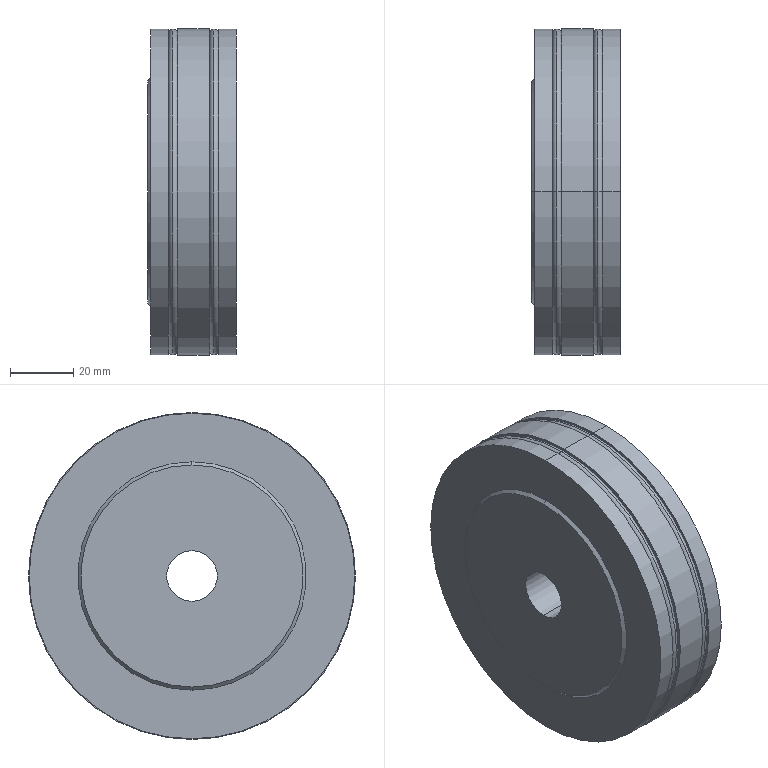Part | SolidWorks | features Sweep 2, Chamfer 1, Revolution 1 | 3 solids | 32 faces | box 28 x 103.442 x 103.442 mm | volume 191573 mm3 | cylinder 12 | plane 8 | torus 8 | cone 4 | commonest cylinder face diameters 97 x4 103 x4 16 x2 103.442 x2
STEP:
#1=CARTESIAN_POINT('',(-24.531,0.,35.124));
#2=VERTEX_POINT('',#1);
#3=CARTESIAN_POINT('',(-24.531,0.,-35.124));
#4=VERTEX_POINT('',#3);
#5=CARTESIAN_POINT('',(-24.531,0.,0.));
#6=DIRECTION('',(-1.,0.,0.));
#7=DIRECTION('',(0.,0.,-1.));
#8=AXIS2_PLACEMENT_3D('',#5,#6,#7);
#9=CIRCLE('',#8,35.124);
#10=EDGE_CURVE('',#2,#4,#9,.T.);
#11=ORIENTED_EDGE('',*,*,#10,.F.);
#12=CARTESIAN_POINT('',(-23.531,0.,36.124));
#13=VERTEX_POINT('',#12);
#14=CARTESIAN_POINT('',(-24.531,0.,35.124));
#15=DIRECTION('',(0.7071,0.,0.7071));
#16=VECTOR('',#15,1000.);
#17=LINE('',#14,#16);
#18=EDGE_CURVE('',#2,#13,#17,.T.);
#19=ORIENTED_EDGE('',*,*,#18,.T.);
#20=CARTESIAN_POINT('',(-23.531,0.,-36.124));
#21=VERTEX_POINT('',#20);
#22=CARTESIAN_POINT('',(-23.531,0.,0.));
#23=DIRECTION('',(-1.,0.,0.));
#24=DIRECTION('',(0.,0.,1.));
#25=AXIS2_PLACEMENT_3D('',#22,#23,#24);
#26=CIRCLE('',#25,36.124);
#27=EDGE_CURVE('',#13,#21,#26,.T.);
#28=ORIENTED_EDGE('',*,*,#27,.T.);
#29=CARTESIAN_POINT('',(-24.531,0.,-35.124));
#30=DIRECTION('',(0.7071,0.,-0.7071));
#31=VECTOR('',#30,1000.);
#32=LINE('',#29,#31);
#33=EDGE_CURVE('',#4,#21,#32,.T.);
#34=ORIENTED_EDGE('',*,*,#33,.F.);
#35=EDGE_LOOP('',(#11,#19,#28,#34));
#36=FACE_OUTER_BOUND('',#35,.T.);
#37=CARTESIAN_POINT('',(-24.531,0.,0.));
#38=DIRECTION('',(1.,0.,0.));
#39=DIRECTION('',(0.,0.,-1.));
#40=AXIS2_PLACEMENT_3D('',#37,#38,#39);
#41=CONICAL_SURFACE('',#40,35.124,0.7854);
#42=ADVANCED_FACE('',(#36),#41,.T.);
#43=CARTESIAN_POINT('',(-10.531,0.,-24.));
#44=VERTEX_POINT('',#43);
#45=CARTESIAN_POINT('',(-10.531,0.,24.));
#46=VERTEX_POINT('',#45);
#47=CARTESIAN_POINT('',(-10.531,0.,0.));
#48=DIRECTION('',(-1.,0.,0.));
#49=DIRECTION('',(0.,0.,1.));
#50=AXIS2_PLACEMENT_3D('',#47,#48,#49);
#51=CIRCLE('',#50,24.);
#52=EDGE_CURVE('',#44,#46,#51,.T.);
#53=ORIENTED_EDGE('',*,*,#52,.T.);
#54=CARTESIAN_POINT('',(3.469,0.,31.5));
#55=VERTEX_POINT('',#54);
#56=CARTESIAN_POINT('',(-10.531,0.,24.));
#57=DIRECTION('',(0.8815,0.,0.4722));
#58=VECTOR('',#57,1000.);
#59=LINE('',#56,#58);
#60=EDGE_CURVE('',#46,#55,#59,.T.);
#61=ORIENTED_EDGE('',*,*,#60,.T.);
#62=CARTESIAN_POINT('',(3.469,0.,-31.5));
#63=VERTEX_POINT('',#62);
#64=CARTESIAN_POINT('',(3.469,0.,0.));
#65=DIRECTION('',(-1.,0.,0.));
#66=DIRECTION('',(0.,0.,1.));
#67=AXIS2_PLACEMENT_3D('',#64,#65,#66);
#68=CIRCLE('',#67,31.5);
#69=EDGE_CURVE('',#63,#55,#68,.T.);
#70=ORIENTED_EDGE('',*,*,#69,.F.);
#71=CARTESIAN_POINT('',(-10.531,0.,-24.));
#72=DIRECTION('',(0.8815,0.,-0.4722));
#73=VECTOR('',#72,1000.);
#74=LINE('',#71,#73);
#75=EDGE_CURVE('',#44,#63,#74,.T.);
#76=ORIENTED_EDGE('',*,*,#75,.F.);
#77=EDGE_LOOP('',(#53,#61,#70,#76));
#78=FACE_OUTER_BOUND('',#77,.T.);
#79=CARTESIAN_POINT('',(-10.531,0.,0.));
#80=DIRECTION('',(1.,0.,0.));
#81=DIRECTION('',(0.,0.,-1.));
#82=AXIS2_PLACEMENT_3D('',#79,#80,#81);
#83=CONICAL_SURFACE('',#82,24.,0.4918);
#84=ADVANCED_FACE('',(#78),#83,.F.);
#85=CARTESIAN_POINT('',(3.469,0.,51.5));
#86=VERTEX_POINT('',#85);
#87=CARTESIAN_POINT('',(3.469,0.,-51.5));
#88=VERTEX_POINT('',#87);
#89=CARTESIAN_POINT('',(3.469,0.,0.));
#90=DIRECTION('',(-1.,0.,0.));
#91=DIRECTION('',(0.,0.,1.));
#92=AXIS2_PLACEMENT_3D('',#89,#90,#91);
#93=CIRCLE('',#92,51.5);
#94=EDGE_CURVE('',#86,#88,#93,.T.);
#95=ORIENTED_EDGE('',*,*,#94,.T.);
#96=CARTESIAN_POINT('',(-2.08,0.,-51.5));
#97=VERTEX_POINT('',#96);
#98=CARTESIAN_POINT('',(-45.717,0.,-51.5));
#99=DIRECTION('',(-1.,0.,0.));
#100=VECTOR('',#99,1000.);
#101=LINE('',#98,#100);
#102=EDGE_CURVE('',#88,#97,#101,.T.);
#103=ORIENTED_EDGE('',*,*,#102,.T.);
#104=CARTESIAN_POINT('',(-2.08,0.,51.5));
#105=VERTEX_POINT('',#104);
#106=CARTESIAN_POINT('',(-2.08,0.,0.));
#107=DIRECTION('',(-1.,0.,0.));
#108=DIRECTION('',(0.,0.,1.));
#109=AXIS2_PLACEMENT_3D('',#106,#107,#108);
#110=CIRCLE('',#109,51.5);
#111=EDGE_CURVE('',#105,#97,#110,.T.);
#112=ORIENTED_EDGE('',*,*,#111,.F.);
#113=CARTESIAN_POINT('',(-45.717,0.,51.5));
#114=DIRECTION('',(-1.,0.,0.));
#115=VECTOR('',#114,1000.);
#116=LINE('',#113,#115);
#117=EDGE_CURVE('',#86,#105,#116,.T.);
#118=ORIENTED_EDGE('',*,*,#117,.F.);
#119=EDGE_LOOP('',(#95,#103,#112,#118));
#120=FACE_OUTER_BOUND('',#119,.T.);
#121=CARTESIAN_POINT('',(-45.717,0.,0.));
#122=DIRECTION('',(-1.,0.,0.));
#123=DIRECTION('',(0.,0.,1.));
#124=AXIS2_PLACEMENT_3D('',#121,#122,#123);
#125=CYLINDRICAL_SURFACE('',#124,51.5);
#126=ADVANCED_FACE('',(#120),#125,.T.);
#127=CARTESIAN_POINT('',(-2.08,0.,48.5));
#128=VERTEX_POINT('',#127);
#129=CARTESIAN_POINT('',(-2.08,0.,-48.5));
#130=VERTEX_POINT('',#129);
#131=CARTESIAN_POINT('',(-2.08,0.,0.));
#132=DIRECTION('',(-1.,0.,0.));
#133=DIRECTION('',(0.,0.,1.));
#134=AXIS2_PLACEMENT_3D('',#131,#132,#133);
#135=CIRCLE('',#134,48.5);
#136=EDGE_CURVE('',#128,#130,#135,.T.);
#137=ORIENTED_EDGE('',*,*,#136,.T.);
#138=CARTESIAN_POINT('',(-5.08,0.,-48.5));
#139=VERTEX_POINT('',#138);
#140=CARTESIAN_POINT('',(-45.717,0.,-48.5));
#141=DIRECTION('',(-1.,0.,0.));
#142=VECTOR('',#141,1000.);
#143=LINE('',#140,#142);
#144=EDGE_CURVE('',#130,#139,#143,.T.);
#145=ORIENTED_EDGE('',*,*,#144,.T.);
#146=CARTESIAN_POINT('',(-5.08,0.,48.5));
#147=VERTEX_POINT('',#146);
#148=CARTESIAN_POINT('',(-5.08,0.,0.));
#149=DIRECTION('',(-1.,0.,0.));
#150=DIRECTION('',(0.,0.,1.));
#151=AXIS2_PLACEMENT_3D('',#148,#149,#150);
#152=CIRCLE('',#151,48.5);
#153=EDGE_CURVE('',#147,#139,#152,.T.);
#154=ORIENTED_EDGE('',*,*,#153,.F.);
#155=CARTESIAN_POINT('',(-45.717,0.,48.5));
#156=DIRECTION('',(-1.,0.,0.));
#157=VECTOR('',#156,1000.);
#158=LINE('',#155,#157);
#159=EDGE_CURVE('',#128,#147,#158,.T.);
#160=ORIENTED_EDGE('',*,*,#159,.F.);
#161=EDGE_LOOP('',(#137,#145,#154,#160));
#162=FACE_OUTER_BOUND('',#161,.T.);
#163=CARTESIAN_POINT('',(-45.717,0.,0.));
#164=DIRECTION('',(-1.,0.,0.));
#165=DIRECTION('',(0.,0.,1.));
#166=AXIS2_PLACEMENT_3D('',#163,#164,#165);
#167=CYLINDRICAL_SURFACE('',#166,48.5);
#168=ADVANCED_FACE('',(#162),#167,.T.);
#169=CARTESIAN_POINT('',(-5.08,0.,51.721));
#170=VERTEX_POINT('',#169);
#171=CARTESIAN_POINT('',(-5.08,0.,-51.721));
#172=VERTEX_POINT('',#171);
#173=CARTESIAN_POINT('',(-5.08,0.,0.));
#174=DIRECTION('',(-1.,0.,0.));
#175=DIRECTION('',(0.,0.,1.));
#176=AXIS2_PLACEMENT_3D('',#173,#174,#175);
#177=CIRCLE('',#176,51.721);
#178=EDGE_CURVE('',#170,#172,#177,.T.);
#179=ORIENTED_EDGE('',*,*,#178,.T.);
#180=CARTESIAN_POINT('',(-15.08,0.,-51.721));
#181=VERTEX_POINT('',#180);
#182=CARTESIAN_POINT('',(-45.717,0.,-51.721));
#183=DIRECTION('',(-1.,0.,0.));
#184=VECTOR('',#183,1000.);
#185=LINE('',#182,#184);
#186=EDGE_CURVE('',#172,#181,#185,.T.);
#187=ORIENTED_EDGE('',*,*,#186,.T.);
#188=CARTESIAN_POINT('',(-15.08,0.,51.721));
#189=VERTEX_POINT('',#188);
#190=CARTESIAN_POINT('',(-15.08,0.,0.));
#191=DIRECTION('',(-1.,0.,0.));
#192=DIRECTION('',(0.,0.,1.));
#193=AXIS2_PLACEMENT_3D('',#190,#191,#192);
#194=CIRCLE('',#193,51.721);
#195=EDGE_CURVE('',#189,#181,#194,.T.);
#196=ORIENTED_EDGE('',*,*,#195,.F.);
#197=CARTESIAN_POINT('',(-45.717,0.,51.721));
#198=DIRECTION('',(-1.,0.,0.));
#199=VECTOR('',#198,1000.);
#200=LINE('',#197,#199);
#201=EDGE_CURVE('',#170,#189,#200,.T.);
#202=ORIENTED_EDGE('',*,*,#201,.F.);
#203=EDGE_LOOP('',(#179,#187,#196,#202));
#204=FACE_OUTER_BOUND('',#203,.T.);
#205=CARTESIAN_POINT('',(-45.717,0.,0.));
#206=DIRECTION('',(-1.,0.,0.));
#207=DIRECTION('',(0.,0.,1.));
#208=AXIS2_PLACEMENT_3D('',#205,#206,#207);
#209=CYLINDRICAL_SURFACE('',#208,51.721);
#210=ADVANCED_FACE('',(#204),#209,.T.);
#211=CARTESIAN_POINT('',(-15.08,0.,48.5));
#212=VERTEX_POINT('',#211);
#213=CARTESIAN_POINT('',(-15.08,0.,-48.5));
#214=VERTEX_POINT('',#213);
#215=CARTESIAN_POINT('',(-15.08,0.,0.));
#216=DIRECTION('',(-1.,0.,0.));
#217=DIRECTION('',(0.,0.,1.));
#218=AXIS2_PLACEMENT_3D('',#215,#216,#217);
#219=CIRCLE('',#218,48.5);
#220=EDGE_CURVE('',#212,#214,#219,.T.);
#221=ORIENTED_EDGE('',*,*,#220,.T.);
#222=CARTESIAN_POINT('',(-18.08,0.,-48.5));
#223=VERTEX_POINT('',#222);
#224=CARTESIAN_POINT('',(-45.717,0.,-48.5));
#225=DIRECTION('',(-1.,0.,0.));
#226=VECTOR('',#225,1000.);
#227=LINE('',#224,#226);
#228=EDGE_CURVE('',#214,#223,#227,.T.);
#229=ORIENTED_EDGE('',*,*,#228,.T.);
#230=CARTESIAN_POINT('',(-18.08,0.,48.5));
#231=VERTEX_POINT('',#230);
#232=CARTESIAN_POINT('',(-18.08,0.,0.));
#233=DIRECTION('',(-1.,0.,0.));
#234=DIRECTION('',(0.,0.,1.));
#235=AXIS2_PLACEMENT_3D('',#232,#233,#234);
#236=CIRCLE('',#235,48.5);
#237=EDGE_CURVE('',#231,#223,#236,.T.);
#238=ORIENTED_EDGE('',*,*,#237,.F.);
#239=CARTESIAN_POINT('',(-45.717,0.,48.5));
#240=DIRECTION('',(-1.,0.,0.));
#241=VECTOR('',#240,1000.);
#242=LINE('',#239,#241);
#243=EDGE_CURVE('',#212,#231,#242,.T.);
#244=ORIENTED_EDGE('',*,*,#243,.F.);
#245=EDGE_LOOP('',(#221,#229,#238,#244));
#246=FACE_OUTER_BOUND('',#245,.T.);
#247=CARTESIAN_POINT('',(-45.717,0.,0.));
#248=DIRECTION('',(-1.,0.,0.));
#249=DIRECTION('',(0.,0.,1.));
#250=AXIS2_PLACEMENT_3D('',#247,#248,#249);
#251=CYLINDRICAL_SURFACE('',#250,48.5);
#252=ADVANCED_FACE('',(#246),#251,.T.);
#253=CARTESIAN_POINT('',(-18.08,0.,51.5));
#254=VERTEX_POINT('',#253);
#255=CARTESIAN_POINT('',(-18.08,0.,-51.5));
#256=VERTEX_POINT('',#255);
#257=CARTESIAN_POINT('',(-18.08,0.,0.));
#258=DIRECTION('',(-1.,0.,0.));
#259=DIRECTION('',(0.,0.,1.));
#260=AXIS2_PLACEMENT_3D('',#257,#258,#259);
#261=CIRCLE('',#260,51.5);
#262=EDGE_CURVE('',#254,#256,#261,.T.);
#263=ORIENTED_EDGE('',*,*,#262,.T.);
#264=CARTESIAN_POINT('',(-23.531,0.,-51.5));
#265=VERTEX_POINT('',#264);
#266=CARTESIAN_POINT('',(-45.717,0.,-51.5));
#267=DIRECTION('',(-1.,0.,0.));
#268=VECTOR('',#267,1000.);
#269=LINE('',#266,#268);
#270=EDGE_CURVE('',#256,#265,#269,.T.);
#271=ORIENTED_EDGE('',*,*,#270,.T.);
#272=CARTESIAN_POINT('',(-23.531,0.,51.5));
#273=VERTEX_POINT('',#272);
#274=CARTESIAN_POINT('',(-23.531,0.,0.));
#275=DIRECTION('',(-1.,0.,0.));
#276=DIRECTION('',(0.,0.,1.));
#277=AXIS2_PLACEMENT_3D('',#274,#275,#276);
#278=CIRCLE('',#277,51.5);
#279=EDGE_CURVE('',#273,#265,#278,.T.);
#280=ORIENTED_EDGE('',*,*,#279,.F.);
#281=CARTESIAN_POINT('',(-45.717,0.,51.5));
#282=DIRECTION('',(-1.,0.,0.));
#283=VECTOR('',#282,1000.);
#284=LINE('',#281,#283);
#285=EDGE_CURVE('',#254,#273,#284,.T.);
#286=ORIENTED_EDGE('',*,*,#285,.F.);
#287=EDGE_LOOP('',(#263,#271,#280,#286));
#288=FACE_OUTER_BOUND('',#287,.T.);
#289=CARTESIAN_POINT('',(-45.717,0.,0.));
#290=DIRECTION('',(-1.,0.,0.));
#291=DIRECTION('',(0.,0.,1.));
#292=AXIS2_PLACEMENT_3D('',#289,#290,#291);
#293=CYLINDRICAL_SURFACE('',#292,51.5);
#294=ADVANCED_FACE('',(#288),#293,.T.);
#295=CARTESIAN_POINT('',(-10.531,0.,-8.));
#296=VERTEX_POINT('',#295);
#297=CARTESIAN_POINT('',(-10.531,0.,8.));
#298=VERTEX_POINT('',#297);
#299=CARTESIAN_POINT('',(-10.531,0.,0.));
#300=DIRECTION('',(-1.,0.,0.));
#301=DIRECTION('',(0.,0.,1.));
#302=AXIS2_PLACEMENT_3D('',#299,#300,#301);
#303=CIRCLE('',#302,8.);
#304=EDGE_CURVE('',#296,#298,#303,.T.);
#305=ORIENTED_EDGE('',*,*,#304,.F.);
#306=CARTESIAN_POINT('',(-24.531,0.,-8.));
#307=VERTEX_POINT('',#306);
#308=CARTESIAN_POINT('',(-45.717,0.,-8.));
#309=DIRECTION('',(-1.,0.,0.));
#310=VECTOR('',#309,1000.);
#311=LINE('',#308,#310);
#312=EDGE_CURVE('',#296,#307,#311,.T.);
#313=ORIENTED_EDGE('',*,*,#312,.T.);
#314=CARTESIAN_POINT('',(-24.531,0.,8.));
#315=VERTEX_POINT('',#314);
#316=CARTESIAN_POINT('',(-24.531,0.,0.));
#317=DIRECTION('',(-1.,0.,0.));
#318=DIRECTION('',(0.,0.,1.));
#319=AXIS2_PLACEMENT_3D('',#316,#317,#318);
#320=CIRCLE('',#319,8.);
#321=EDGE_CURVE('',#307,#315,#320,.T.);
#322=ORIENTED_EDGE('',*,*,#321,.T.);
#323=CARTESIAN_POINT('',(-45.717,0.,8.));
#324=DIRECTION('',(-1.,0.,0.));
#325=VECTOR('',#324,1000.);
#326=LINE('',#323,#325);
#327=EDGE_CURVE('',#298,#315,#326,.T.);
#328=ORIENTED_EDGE('',*,*,#327,.F.);
#329=EDGE_LOOP('',(#305,#313,#322,#328));
#330=FACE_OUTER_BOUND('',#329,.T.);
#331=CARTESIAN_POINT('',(-45.717,0.,0.));
#332=DIRECTION('',(-1.,0.,0.));
#333=DIRECTION('',(0.,0.,1.));
#334=AXIS2_PLACEMENT_3D('',#331,#332,#333);
#335=CYLINDRICAL_SURFACE('',#334,8.);
#336=ADVANCED_FACE('',(#330),#335,.F.);
#337=ORIENTED_EDGE('',*,*,#312,.F.);
#338=CARTESIAN_POINT('',(-10.531,0.,0.));
#339=DIRECTION('',(-1.,0.,0.));
#340=DIRECTION('',(0.,0.,1.));
#341=AXIS2_PLACEMENT_3D('',#338,#339,#340);
#342=CIRCLE('',#341,8.);
#343=EDGE_CURVE('',#298,#296,#342,.T.);
#344=ORIENTED_EDGE('',*,*,#343,.F.);
#345=ORIENTED_EDGE('',*,*,#327,.T.);
#346=CARTESIAN_POINT('',(-24.531,0.,0.));
#347=DIRECTION('',(-1.,0.,0.));
#348=DIRECTION('',(0.,0.,1.));
#349=AXIS2_PLACEMENT_3D('',#346,#347,#348);
#350=CIRCLE('',#349,8.);
#351=EDGE_CURVE('',#315,#307,#350,.T.);
#352=ORIENTED_EDGE('',*,*,#351,.T.);
#353=EDGE_LOOP('',(#337,#344,#345,#352));
#354=FACE_OUTER_BOUND('',#353,.T.);
#355=CARTESIAN_POINT('',(-45.717,0.,0.));
#356=DIRECTION('',(-1.,0.,0.));
#357=DIRECTION('',(0.,0.,1.));
#358=AXIS2_PLACEMENT_3D('',#355,#356,#357);
#359=CYLINDRICAL_SURFACE('',#358,8.);
#360=ADVANCED_FACE('',(#354),#359,.F.);
#361=CARTESIAN_POINT('',(-24.531,0.,0.));
#362=DIRECTION('',(-1.,0.,0.));
#363=DIRECTION('',(0.,0.,-1.));
#364=AXIS2_PLACEMENT_3D('',#361,#362,#363);
#365=CIRCLE('',#364,35.124);
#366=EDGE_CURVE('',#4,#2,#365,.T.);
#367=ORIENTED_EDGE('',*,*,#366,.T.);
#368=ORIENTED_EDGE('',*,*,#10,.T.);
#369=EDGE_LOOP('',(#367,#368));
#370=FACE_OUTER_BOUND('',#369,.T.);
#371=ORIENTED_EDGE('',*,*,#351,.F.);
#372=ORIENTED_EDGE('',*,*,#321,.F.);
#373=EDGE_LOOP('',(#371,#372));
#374=FACE_BOUND('',#373,.T.);
#375=CARTESIAN_POINT('',(-24.531,8.,0.));
#376=DIRECTION('',(1.,0.,0.));
#377=DIRECTION('',(0.,0.,-1.));
#378=AXIS2_PLACEMENT_3D('',#375,#376,#377);
#379=PLANE('',#378);
#380=ADVANCED_FACE('',(#370,#374),#379,.F.);
#381=CARTESIAN_POINT('',(-23.531,0.,0.));
#382=DIRECTION('',(-1.,0.,0.));
#383=DIRECTION('',(0.,0.,1.));
#384=AXIS2_PLACEMENT_3D('',#381,#382,#383);
#385=CIRCLE('',#384,36.124);
#386=EDGE_CURVE('',#21,#13,#385,.T.);
#387=ORIENTED_EDGE('',*,*,#386,.F.);
#388=ORIENTED_EDGE('',*,*,#27,.F.);
#389=EDGE_LOOP('',(#387,#388));
#390=FACE_BOUND('',#389,.T.);
#391=ORIENTED_EDGE('',*,*,#279,.T.);
#392=CARTESIAN_POINT('',(-23.531,0.,0.));
#393=DIRECTION('',(-1.,0.,0.));
#394=DIRECTION('',(0.,0.,1.));
#395=AXIS2_PLACEMENT_3D('',#392,#393,#394);
#396=CIRCLE('',#395,51.5);
#397=EDGE_CURVE('',#265,#273,#396,.T.);
#398=ORIENTED_EDGE('',*,*,#397,.T.);
#399=EDGE_LOOP('',(#391,#398));
#400=FACE_OUTER_BOUND('',#399,.T.);
#401=CARTESIAN_POINT('',(-23.531,36.124,0.));
#402=DIRECTION('',(1.,0.,0.));
#403=DIRECTION('',(0.,0.,-1.));
#404=AXIS2_PLACEMENT_3D('',#401,#402,#403);
#405=PLANE('',#404);
#406=ADVANCED_FACE('',(#390,#400),#405,.F.);
#407=ORIENTED_EDGE('',*,*,#270,.F.);
#408=CARTESIAN_POINT('',(-18.08,0.,0.));
#409=DIRECTION('',(-1.,0.,0.));
#410=DIRECTION('',(0.,0.,1.));
#411=AXIS2_PLACEMENT_3D('',#408,#409,#410);
#412=CIRCLE('',#411,51.5);
#413=EDGE_CURVE('',#256,#254,#412,.T.);
#414=ORIENTED_EDGE('',*,*,#413,.T.);
#415=ORIENTED_EDGE('',*,*,#285,.T.);
#416=ORIENTED_EDGE('',*,*,#397,.F.);
#417=EDGE_LOOP('',(#407,#414,#415,#416));
#418=FACE_OUTER_BOUND('',#417,.T.);
#419=CARTESIAN_POINT('',(-45.717,0.,0.));
#420=DIRECTION('',(-1.,0.,0.));
#421=DIRECTION('',(0.,0.,1.));
#422=AXIS2_PLACEMENT_3D('',#419,#420,#421);
#423=CYLINDRICAL_SURFACE('',#422,51.5);
#424=ADVANCED_FACE('',(#418),#423,.T.);
#425=ORIENTED_EDGE('',*,*,#262,.F.);
#426=ORIENTED_EDGE('',*,*,#413,.F.);
#427=EDGE_LOOP('',(#425,#426));
#428=FACE_OUTER_BOUND('',#427,.T.);
#429=ORIENTED_EDGE('',*,*,#237,.T.);
#430=CARTESIAN_POINT('',(-18.08,0.,0.));
#431=DIRECTION('',(-1.,0.,0.));
#432=DIRECTION('',(0.,0.,1.));
#433=AXIS2_PLACEMENT_3D('',#430,#431,#432);
#434=CIRCLE('',#433,48.5);
#435=EDGE_CURVE('',#223,#231,#434,.T.);
#436=ORIENTED_EDGE('',*,*,#435,.T.);
#437=EDGE_LOOP('',(#429,#436));
#438=FACE_BOUND('',#437,.T.);
#439=CARTESIAN_POINT('',(-18.08,51.5,0.));
#440=DIRECTION('',(-1.,0.,0.));
#441=DIRECTION('',(0.,0.,1.));
#442=AXIS2_PLACEMENT_3D('',#439,#440,#441);
#443=PLANE('',#442);
#444=ADVANCED_FACE('',(#428,#438),#443,.F.);
#445=ORIENTED_EDGE('',*,*,#228,.F.);
#446=CARTESIAN_POINT('',(-15.08,0.,0.));
#447=DIRECTION('',(-1.,0.,0.));
#448=DIRECTION('',(0.,0.,1.));
#449=AXIS2_PLACEMENT_3D('',#446,#447,#448);
#450=CIRCLE('',#449,48.5);
#451=EDGE_CURVE('',#214,#212,#450,.T.);
#452=ORIENTED_EDGE('',*,*,#451,.T.);
#453=ORIENTED_EDGE('',*,*,#243,.T.);
#454=ORIENTED_EDGE('',*,*,#435,.F.);
#455=EDGE_LOOP('',(#445,#452,#453,#454));
#456=FACE_OUTER_BOUND('',#455,.T.);
#457=CARTESIAN_POINT('',(-45.717,0.,0.));
#458=DIRECTION('',(-1.,0.,0.));
#459=DIRECTION('',(0.,0.,1.));
#460=AXIS2_PLACEMENT_3D('',#457,#458,#459);
#461=CYLINDRICAL_SURFACE('',#460,48.5);
#462=ADVANCED_FACE('',(#456),#461,.T.);
#463=ORIENTED_EDGE('',*,*,#195,.T.);
#464=CARTESIAN_POINT('',(-15.08,0.,0.));
#465=DIRECTION('',(-1.,0.,0.));
#466=DIRECTION('',(0.,0.,1.));
#467=AXIS2_PLACEMENT_3D('',#464,#465,#466);
#468=CIRCLE('',#467,51.721);
#469=EDGE_CURVE('',#181,#189,#468,.T.);
#470=ORIENTED_EDGE('',*,*,#469,.T.);
#471=EDGE_LOOP('',(#463,#470));
#472=FACE_OUTER_BOUND('',#471,.T.);
#473=ORIENTED_EDGE('',*,*,#220,.F.);
#474=ORIENTED_EDGE('',*,*,#451,.F.);
#475=EDGE_LOOP('',(#473,#474));
#476=FACE_BOUND('',#475,.T.);
#477=CARTESIAN_POINT('',(-15.08,48.5,0.));
#478=DIRECTION('',(1.,0.,0.));
#479=DIRECTION('',(0.,0.,-1.));
#480=AXIS2_PLACEMENT_3D('',#477,#478,#479);
#481=PLANE('',#480);
#482=ADVANCED_FACE('',(#472,#476),#481,.F.);
#483=ORIENTED_EDGE('',*,*,#186,.F.);
#484=CARTESIAN_POINT('',(-5.08,0.,0.));
#485=DIRECTION('',(-1.,0.,0.));
#486=DIRECTION('',(0.,0.,1.));
#487=AXIS2_PLACEMENT_3D('',#484,#485,#486);
#488=CIRCLE('',#487,51.721);
#489=EDGE_CURVE('',#172,#170,#488,.T.);
#490=ORIENTED_EDGE('',*,*,#489,.T.);
#491=ORIENTED_EDGE('',*,*,#201,.T.);
#492=ORIENTED_EDGE('',*,*,#469,.F.);
#493=EDGE_LOOP('',(#483,#490,#491,#492));
#494=FACE_OUTER_BOUND('',#493,.T.);
#495=CARTESIAN_POINT('',(-45.717,0.,0.));
#496=DIRECTION('',(-1.,0.,0.));
#497=DIRECTION('',(0.,0.,1.));
#498=AXIS2_PLACEMENT_3D('',#495,#496,#497);
#499=CYLINDRICAL_SURFACE('',#498,51.721);
#500=ADVANCED_FACE('',(#494),#499,.T.);
#501=ORIENTED_EDGE('',*,*,#178,.F.);
#502=ORIENTED_EDGE('',*,*,#489,.F.);
#503=EDGE_LOOP('',(#501,#502));
#504=FACE_OUTER_BOUND('',#503,.T.);
#505=ORIENTED_EDGE('',*,*,#153,.T.);
#506=CARTESIAN_POINT('',(-5.08,0.,0.));
#507=DIRECTION('',(-1.,0.,0.));
#508=DIRECTION('',(0.,0.,1.));
#509=AXIS2_PLACEMENT_3D('',#506,#507,#508);
#510=CIRCLE('',#509,48.5);
#511=EDGE_CURVE('',#139,#147,#510,.T.);
#512=ORIENTED_EDGE('',*,*,#511,.T.);
#513=EDGE_LOOP('',(#505,#512));
#514=FACE_BOUND('',#513,.T.);
#515=CARTESIAN_POINT('',(-5.08,51.721,0.));
#516=DIRECTION('',(-1.,0.,0.));
#517=DIRECTION('',(0.,0.,1.));
#518=AXIS2_PLACEMENT_3D('',#515,#516,#517);
#519=PLANE('',#518);
#520=ADVANCED_FACE('',(#504,#514),#519,.F.);
#521=ORIENTED_EDGE('',*,*,#144,.F.);
#522=CARTESIAN_POINT('',(-2.08,0.,0.));
#523=DIRECTION('',(-1.,0.,0.));
#524=DIRECTION('',(0.,0.,1.));
#525=AXIS2_PLACEMENT_3D('',#522,#523,#524);
#526=CIRCLE('',#525,48.5);
#527=EDGE_CURVE('',#130,#128,#526,.T.);
#528=ORIENTED_EDGE('',*,*,#527,.T.);
#529=ORIENTED_EDGE('',*,*,#159,.T.);
#530=ORIENTED_EDGE('',*,*,#511,.F.);
#531=EDGE_LOOP('',(#521,#528,#529,#530));
#532=FACE_OUTER_BOUND('',#531,.T.);
#533=CARTESIAN_POINT('',(-45.717,0.,0.));
#534=DIRECTION('',(-1.,0.,0.));
#535=DIRECTION('',(0.,0.,1.));
#536=AXIS2_PLACEMENT_3D('',#533,#534,#535);
#537=CYLINDRICAL_SURFACE('',#536,48.5);
#538=ADVANCED_FACE('',(#532),#537,.T.);
#539=ORIENTED_EDGE('',*,*,#111,.T.);
#540=CARTESIAN_POINT('',(-2.08,0.,0.));
#541=DIRECTION('',(-1.,0.,0.));
#542=DIRECTION('',(0.,0.,1.));
#543=AXIS2_PLACEMENT_3D('',#540,#541,#542);
#544=CIRCLE('',#543,51.5);
#545=EDGE_CURVE('',#97,#105,#544,.T.);
#546=ORIENTED_EDGE('',*,*,#545,.T.);
#547=EDGE_LOOP('',(#539,#546));
#548=FACE_OUTER_BOUND('',#547,.T.);
#549=ORIENTED_EDGE('',*,*,#136,.F.);
#550=ORIENTED_EDGE('',*,*,#527,.F.);
#551=EDGE_LOOP('',(#549,#550));
#552=FACE_BOUND('',#551,.T.);
#553=CARTESIAN_POINT('',(-2.08,48.5,0.));
#554=DIRECTION('',(1.,0.,0.));
#555=DIRECTION('',(0.,0.,-1.));
#556=AXIS2_PLACEMENT_3D('',#553,#554,#555);
#557=PLANE('',#556);
#558=ADVANCED_FACE('',(#548,#552),#557,.F.);
#559=ORIENTED_EDGE('',*,*,#102,.F.);
#560=CARTESIAN_POINT('',(3.469,0.,0.));
#561=DIRECTION('',(-1.,0.,0.));
#562=DIRECTION('',(0.,0.,1.));
#563=AXIS2_PLACEMENT_3D('',#560,#561,#562);
#564=CIRCLE('',#563,51.5);
#565=EDGE_CURVE('',#88,#86,#564,.T.);
#566=ORIENTED_EDGE('',*,*,#565,.T.);
#567=ORIENTED_EDGE('',*,*,#117,.T.);
#568=ORIENTED_EDGE('',*,*,#545,.F.);
#569=EDGE_LOOP('',(#559,#566,#567,#568));
#570=FACE_OUTER_BOUND('',#569,.T.);
#571=CARTESIAN_POINT('',(-45.717,0.,0.));
#572=DIRECTION('',(-1.,0.,0.));
#573=DIRECTION('',(0.,0.,1.));
#574=AXIS2_PLACEMENT_3D('',#571,#572,#573);
#575=CYLINDRICAL_SURFACE('',#574,51.5);
#576=ADVANCED_FACE('',(#570),#575,.T.);
#577=ORIENTED_EDGE('',*,*,#94,.F.);
#578=ORIENTED_EDGE('',*,*,#565,.F.);
#579=EDGE_LOOP('',(#577,#578));
#580=FACE_OUTER_BOUND('',#579,.T.);
#581=ORIENTED_EDGE('',*,*,#69,.T.);
#582=CARTESIAN_POINT('',(3.469,0.,0.));
#583=DIRECTION('',(-1.,0.,0.));
#584=DIRECTION('',(0.,0.,1.));
#585=AXIS2_PLACEMENT_3D('',#582,#583,#584);
#586=CIRCLE('',#585,31.5);
#587=EDGE_CURVE('',#55,#63,#586,.T.);
#588=ORIENTED_EDGE('',*,*,#587,.T.);
#589=EDGE_LOOP('',(#581,#588));
#590=FACE_BOUND('',#589,.T.);
#591=CARTESIAN_POINT('',(3.469,51.5,0.));
#592=DIRECTION('',(-1.,0.,0.));
#593=DIRECTION('',(0.,0.,1.));
#594=AXIS2_PLACEMENT_3D('',#591,#592,#593);
#595=PLANE('',#594);
#596=ADVANCED_FACE('',(#580,#590),#595,.F.);
#597=ORIENTED_EDGE('',*,*,#60,.F.);
#598=CARTESIAN_POINT('',(-10.531,0.,0.));
#599=DIRECTION('',(-1.,0.,0.));
#600=DIRECTION('',(0.,0.,1.));
#601=AXIS2_PLACEMENT_3D('',#598,#599,#600);
#602=CIRCLE('',#601,24.);
#603=EDGE_CURVE('',#46,#44,#602,.T.);
#604=ORIENTED_EDGE('',*,*,#603,.T.);
#605=ORIENTED_EDGE('',*,*,#75,.T.);
#606=ORIENTED_EDGE('',*,*,#587,.F.);
#607=EDGE_LOOP('',(#597,#604,#605,#606));
#608=FACE_OUTER_BOUND('',#607,.T.);
#609=CARTESIAN_POINT('',(-10.531,0.,0.));
#610=DIRECTION('',(1.,0.,0.));
#611=DIRECTION('',(0.,0.,-1.));
#612=AXIS2_PLACEMENT_3D('',#609,#610,#611);
#613=CONICAL_SURFACE('',#612,24.,0.4918);
#614=ADVANCED_FACE('',(#608),#613,.F.);
#615=ORIENTED_EDGE('',*,*,#52,.F.);
#616=ORIENTED_EDGE('',*,*,#603,.F.);
#617=EDGE_LOOP('',(#615,#616));
#618=FACE_OUTER_BOUND('',#617,.T.);
#619=ORIENTED_EDGE('',*,*,#343,.T.);
#620=ORIENTED_EDGE('',*,*,#304,.T.);
#621=EDGE_LOOP('',(#619,#620));
#622=FACE_BOUND('',#621,.T.);
#623=CARTESIAN_POINT('',(-10.531,24.,0.));
#624=DIRECTION('',(-1.,0.,0.));
#625=DIRECTION('',(0.,0.,1.));
#626=AXIS2_PLACEMENT_3D('',#623,#624,#625);
#627=PLANE('',#626);
#628=ADVANCED_FACE('',(#618,#622),#627,.F.);
#629=ORIENTED_EDGE('',*,*,#18,.F.);
#630=ORIENTED_EDGE('',*,*,#366,.F.);
#631=ORIENTED_EDGE('',*,*,#33,.T.);
#632=ORIENTED_EDGE('',*,*,#386,.T.);
#633=EDGE_LOOP('',(#629,#630,#631,#632));
#634=FACE_OUTER_BOUND('',#633,.T.);
#635=CARTESIAN_POINT('',(-24.531,0.,0.));
#636=DIRECTION('',(1.,0.,0.));
#637=DIRECTION('',(0.,0.,-1.));
#638=AXIS2_PLACEMENT_3D('',#635,#636,#637);
#639=CONICAL_SURFACE('',#638,35.124,0.7854);
#640=ADVANCED_FACE('',(#634),#639,.T.);
#641=CLOSED_SHELL('',(#42,#84,#126,#168,#210,#252,#294,#336,#360,#380,#406,#424,#444,#462,#482,#500,#520,#538,#558,#576,#596,#614,#628,#640));
#642=MANIFOLD_SOLID_BREP('',#641);
#643=CARTESIAN_POINT('',(-3.58,0.,51.5));
#644=VERTEX_POINT('',#643);
#645=CARTESIAN_POINT('',(-3.58,0.,48.5));
#646=VERTEX_POINT('',#645);
#647=CARTESIAN_POINT('',(-3.58,0.,50.));
#648=DIRECTION('',(0.,1.,0.));
#649=DIRECTION('',(0.,0.,1.));
#650=AXIS2_PLACEMENT_3D('',#647,#648,#649);
#651=CIRCLE('',#650,1.5);
#652=EDGE_CURVE('',#644,#646,#651,.T.);
#653=ORIENTED_EDGE('',*,*,#652,.F.);
#654=CARTESIAN_POINT('',(-3.58,0.,-51.5));
#655=VERTEX_POINT('',#654);
#656=CARTESIAN_POINT('',(-3.58,0.,0.));
#657=DIRECTION('',(1.,0.,0.));
#658=DIRECTION('',(0.,0.,-1.));
#659=AXIS2_PLACEMENT_3D('',#656,#657,#658);
#660=CIRCLE('',#659,51.5);
#661=EDGE_CURVE('',#644,#655,#660,.T.);
#662=ORIENTED_EDGE('',*,*,#661,.T.);
#663=CARTESIAN_POINT('',(-3.58,0.,-48.5));
#664=VERTEX_POINT('',#663);
#665=CARTESIAN_POINT('',(-3.58,0.,-50.));
#666=DIRECTION('',(0.,-1.,0.));
#667=DIRECTION('',(0.,0.,-1.));
#668=AXIS2_PLACEMENT_3D('',#665,#666,#667);
#669=CIRCLE('',#668,1.5);
#670=EDGE_CURVE('',#655,#664,#669,.T.);
#671=ORIENTED_EDGE('',*,*,#670,.T.);
#672=CARTESIAN_POINT('',(-3.58,0.,0.));
#673=DIRECTION('',(1.,0.,0.));
#674=DIRECTION('',(0.,0.,-1.));
#675=AXIS2_PLACEMENT_3D('',#672,#673,#674);
#676=CIRCLE('',#675,48.5);
#677=EDGE_CURVE('',#646,#664,#676,.T.);
#678=ORIENTED_EDGE('',*,*,#677,.F.);
#679=EDGE_LOOP('',(#653,#662,#671,#678));
#680=FACE_OUTER_BOUND('',#679,.T.);
#681=CARTESIAN_POINT('',(-3.58,0.,0.));
#682=DIRECTION('',(1.,0.,0.));
#683=DIRECTION('',(0.,0.,-1.));
#684=AXIS2_PLACEMENT_3D('',#681,#682,#683);
#685=TOROIDAL_SURFACE('',#684,50.,1.5);
#686=ADVANCED_FACE('',(#680),#685,.T.);
#687=ORIENTED_EDGE('',*,*,#670,.F.);
#688=CARTESIAN_POINT('',(-3.58,0.,0.));
#689=DIRECTION('',(1.,0.,0.));
#690=DIRECTION('',(0.,0.,-1.));
#691=AXIS2_PLACEMENT_3D('',#688,#689,#690);
#692=CIRCLE('',#691,51.5);
#693=EDGE_CURVE('',#655,#644,#692,.T.);
#694=ORIENTED_EDGE('',*,*,#693,.T.);
#695=ORIENTED_EDGE('',*,*,#652,.T.);
#696=CARTESIAN_POINT('',(-3.58,0.,0.));
#697=DIRECTION('',(1.,0.,0.));
#698=DIRECTION('',(0.,0.,-1.));
#699=AXIS2_PLACEMENT_3D('',#696,#697,#698);
#700=CIRCLE('',#699,48.5);
#701=EDGE_CURVE('',#664,#646,#700,.T.);
#702=ORIENTED_EDGE('',*,*,#701,.F.);
#703=EDGE_LOOP('',(#687,#694,#695,#702));
#704=FACE_OUTER_BOUND('',#703,.T.);
#705=CARTESIAN_POINT('',(-3.58,0.,0.));
#706=DIRECTION('',(1.,0.,0.));
#707=DIRECTION('',(0.,0.,-1.));
#708=AXIS2_PLACEMENT_3D('',#705,#706,#707);
#709=TOROIDAL_SURFACE('',#708,50.,1.5);
#710=ADVANCED_FACE('',(#704),#709,.T.);
#711=ORIENTED_EDGE('',*,*,#693,.F.);
#712=CARTESIAN_POINT('',(-3.58,0.,-50.));
#713=DIRECTION('',(0.,-1.,0.));
#714=DIRECTION('',(0.,0.,-1.));
#715=AXIS2_PLACEMENT_3D('',#712,#713,#714);
#716=CIRCLE('',#715,1.5);
#717=EDGE_CURVE('',#664,#655,#716,.T.);
#718=ORIENTED_EDGE('',*,*,#717,.F.);
#719=ORIENTED_EDGE('',*,*,#701,.T.);
#720=CARTESIAN_POINT('',(-3.58,0.,50.));
#721=DIRECTION('',(0.,1.,0.));
#722=DIRECTION('',(0.,0.,1.));
#723=AXIS2_PLACEMENT_3D('',#720,#721,#722);
#724=CIRCLE('',#723,1.5);
#725=EDGE_CURVE('',#646,#644,#724,.T.);
#726=ORIENTED_EDGE('',*,*,#725,.T.);
#727=EDGE_LOOP('',(#711,#718,#719,#726));
#728=FACE_OUTER_BOUND('',#727,.T.);
#729=CARTESIAN_POINT('',(-3.58,0.,0.));
#730=DIRECTION('',(1.,0.,0.));
#731=DIRECTION('',(0.,0.,-1.));
#732=AXIS2_PLACEMENT_3D('',#729,#730,#731);
#733=TOROIDAL_SURFACE('',#732,50.,1.5);
#734=ADVANCED_FACE('',(#728),#733,.T.);
#735=ORIENTED_EDGE('',*,*,#661,.F.);
#736=ORIENTED_EDGE('',*,*,#725,.F.);
#737=ORIENTED_EDGE('',*,*,#677,.T.);
#738=ORIENTED_EDGE('',*,*,#717,.T.);
#739=EDGE_LOOP('',(#735,#736,#737,#738));
#740=FACE_OUTER_BOUND('',#739,.T.);
#741=CARTESIAN_POINT('',(-3.58,0.,0.));
#742=DIRECTION('',(1.,0.,0.));
#743=DIRECTION('',(0.,0.,-1.));
#744=AXIS2_PLACEMENT_3D('',#741,#742,#743);
#745=TOROIDAL_SURFACE('',#744,50.,1.5);
#746=ADVANCED_FACE('',(#740),#745,.T.);
#747=CLOSED_SHELL('',(#686,#710,#734,#746));
#748=MANIFOLD_SOLID_BREP('',#747);
#749=CARTESIAN_POINT('',(-16.58,0.,51.5));
#750=VERTEX_POINT('',#749);
#751=CARTESIAN_POINT('',(-16.58,0.,48.5));
#752=VERTEX_POINT('',#751);
#753=CARTESIAN_POINT('',(-16.58,0.,50.));
#754=DIRECTION('',(0.,1.,0.));
#755=DIRECTION('',(0.,0.,1.));
#756=AXIS2_PLACEMENT_3D('',#753,#754,#755);
#757=CIRCLE('',#756,1.5);
#758=EDGE_CURVE('',#750,#752,#757,.T.);
#759=ORIENTED_EDGE('',*,*,#758,.F.);
#760=CARTESIAN_POINT('',(-16.58,0.,-51.5));
#761=VERTEX_POINT('',#760);
#762=CARTESIAN_POINT('',(-16.58,0.,0.));
#763=DIRECTION('',(1.,0.,0.));
#764=DIRECTION('',(0.,0.,-1.));
#765=AXIS2_PLACEMENT_3D('',#762,#763,#764);
#766=CIRCLE('',#765,51.5);
#767=EDGE_CURVE('',#750,#761,#766,.T.);
#768=ORIENTED_EDGE('',*,*,#767,.T.);
#769=CARTESIAN_POINT('',(-16.58,0.,-48.5));
#770=VERTEX_POINT('',#769);
#771=CARTESIAN_POINT('',(-16.58,0.,-50.));
#772=DIRECTION('',(0.,-1.,0.));
#773=DIRECTION('',(0.,0.,-1.));
#774=AXIS2_PLACEMENT_3D('',#771,#772,#773);
#775=CIRCLE('',#774,1.5);
#776=EDGE_CURVE('',#761,#770,#775,.T.);
#777=ORIENTED_EDGE('',*,*,#776,.T.);
#778=CARTESIAN_POINT('',(-16.58,0.,0.));
#779=DIRECTION('',(1.,0.,0.));
#780=DIRECTION('',(0.,0.,-1.));
#781=AXIS2_PLACEMENT_3D('',#778,#779,#780);
#782=CIRCLE('',#781,48.5);
#783=EDGE_CURVE('',#752,#770,#782,.T.);
#784=ORIENTED_EDGE('',*,*,#783,.F.);
#785=EDGE_LOOP('',(#759,#768,#777,#784));
#786=FACE_OUTER_BOUND('',#785,.T.);
#787=CARTESIAN_POINT('',(-16.58,0.,0.));
#788=DIRECTION('',(1.,0.,0.));
#789=DIRECTION('',(0.,0.,-1.));
#790=AXIS2_PLACEMENT_3D('',#787,#788,#789);
#791=TOROIDAL_SURFACE('',#790,50.,1.5);
#792=ADVANCED_FACE('',(#786),#791,.T.);
#793=ORIENTED_EDGE('',*,*,#776,.F.);
#794=CARTESIAN_POINT('',(-16.58,0.,0.));
#795=DIRECTION('',(1.,0.,0.));
#796=DIRECTION('',(0.,0.,-1.));
#797=AXIS2_PLACEMENT_3D('',#794,#795,#796);
#798=CIRCLE('',#797,51.5);
#799=EDGE_CURVE('',#761,#750,#798,.T.);
#800=ORIENTED_EDGE('',*,*,#799,.T.);
#801=ORIENTED_EDGE('',*,*,#758,.T.);
#802=CARTESIAN_POINT('',(-16.58,0.,0.));
#803=DIRECTION('',(1.,0.,0.));
#804=DIRECTION('',(0.,0.,-1.));
#805=AXIS2_PLACEMENT_3D('',#802,#803,#804);
#806=CIRCLE('',#805,48.5);
#807=EDGE_CURVE('',#770,#752,#806,.T.);
#808=ORIENTED_EDGE('',*,*,#807,.F.);
#809=EDGE_LOOP('',(#793,#800,#801,#808));
#810=FACE_OUTER_BOUND('',#809,.T.);
#811=CARTESIAN_POINT('',(-16.58,0.,0.));
#812=DIRECTION('',(1.,0.,0.));
#813=DIRECTION('',(0.,0.,-1.));
#814=AXIS2_PLACEMENT_3D('',#811,#812,#813);
#815=TOROIDAL_SURFACE('',#814,50.,1.5);
#816=ADVANCED_FACE('',(#810),#815,.T.);
#817=ORIENTED_EDGE('',*,*,#799,.F.);
#818=CARTESIAN_POINT('',(-16.58,0.,-50.));
#819=DIRECTION('',(0.,-1.,0.));
#820=DIRECTION('',(0.,0.,-1.));
#821=AXIS2_PLACEMENT_3D('',#818,#819,#820);
#822=CIRCLE('',#821,1.5);
#823=EDGE_CURVE('',#770,#761,#822,.T.);
#824=ORIENTED_EDGE('',*,*,#823,.F.);
#825=ORIENTED_EDGE('',*,*,#807,.T.);
#826=CARTESIAN_POINT('',(-16.58,0.,50.));
#827=DIRECTION('',(0.,1.,0.));
#828=DIRECTION('',(0.,0.,1.));
#829=AXIS2_PLACEMENT_3D('',#826,#827,#828);
#830=CIRCLE('',#829,1.5);
#831=EDGE_CURVE('',#752,#750,#830,.T.);
#832=ORIENTED_EDGE('',*,*,#831,.T.);
#833=EDGE_LOOP('',(#817,#824,#825,#832));
#834=FACE_OUTER_BOUND('',#833,.T.);
#835=CARTESIAN_POINT('',(-16.58,0.,0.));
#836=DIRECTION('',(1.,0.,0.));
#837=DIRECTION('',(0.,0.,-1.));
#838=AXIS2_PLACEMENT_3D('',#835,#836,#837);
#839=TOROIDAL_SURFACE('',#838,50.,1.5);
#840=ADVANCED_FACE('',(#834),#839,.T.);
#841=ORIENTED_EDGE('',*,*,#767,.F.);
#842=ORIENTED_EDGE('',*,*,#831,.F.);
#843=ORIENTED_EDGE('',*,*,#783,.T.);
#844=ORIENTED_EDGE('',*,*,#823,.T.);
#845=EDGE_LOOP('',(#841,#842,#843,#844));
#846=FACE_OUTER_BOUND('',#845,.T.);
#847=CARTESIAN_POINT('',(-16.58,0.,0.));
#848=DIRECTION('',(1.,0.,0.));
#849=DIRECTION('',(0.,0.,-1.));
#850=AXIS2_PLACEMENT_3D('',#847,#848,#849);
#851=TOROIDAL_SURFACE('',#850,50.,1.5);
#852=ADVANCED_FACE('',(#846),#851,.T.);
#853=CLOSED_SHELL('',(#792,#816,#840,#852));
#854=MANIFOLD_SOLID_BREP('',#853);
#855=CARTESIAN_POINT('',(0.,0.,0.));
#856=DIRECTION('',(0.,0.,1.));
#857=DIRECTION('',(1.,0.,0.));
#858=AXIS2_PLACEMENT_3D('',#855,#856,#857);
#859=(LENGTH_UNIT()NAMED_UNIT(*)SI_UNIT(.MILLI.,.METRE.));
#860=UNCERTAINTY_MEASURE_WITH_UNIT(LENGTH_MEASURE(0.00001),#859,'','');
#861=(NAMED_UNIT(*)PLANE_ANGLE_UNIT()SI_UNIT($,.RADIAN.));
#862=(NAMED_UNIT(*)SI_UNIT($,.STERADIAN.)SOLID_ANGLE_UNIT());
#863=(GEOMETRIC_REPRESENTATION_CONTEXT(3)GLOBAL_UNCERTAINTY_ASSIGNED_CONTEXT((#860))GLOBAL_UNIT_ASSIGNED_CONTEXT((#859,#861,#862))REPRESENTATION_CONTEXT('',''));
#864=ADVANCED_BREP_SHAPE_REPRESENTATION('',(#642,#748,#854,#858),#863);